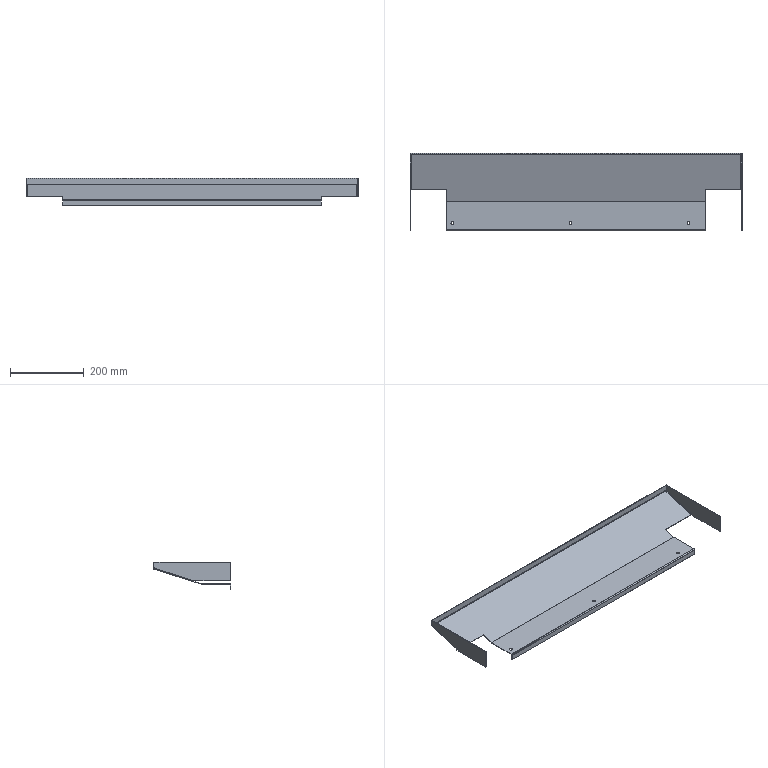Part | NX | features solid 2 | 1 solid | 66 faces | box 900 x 209.5 x 75 mm | volume 320620 mm3 | plane 50 | cylinder 16 | commonest cylinder face diameters 8 x6 3 x5 6 x5